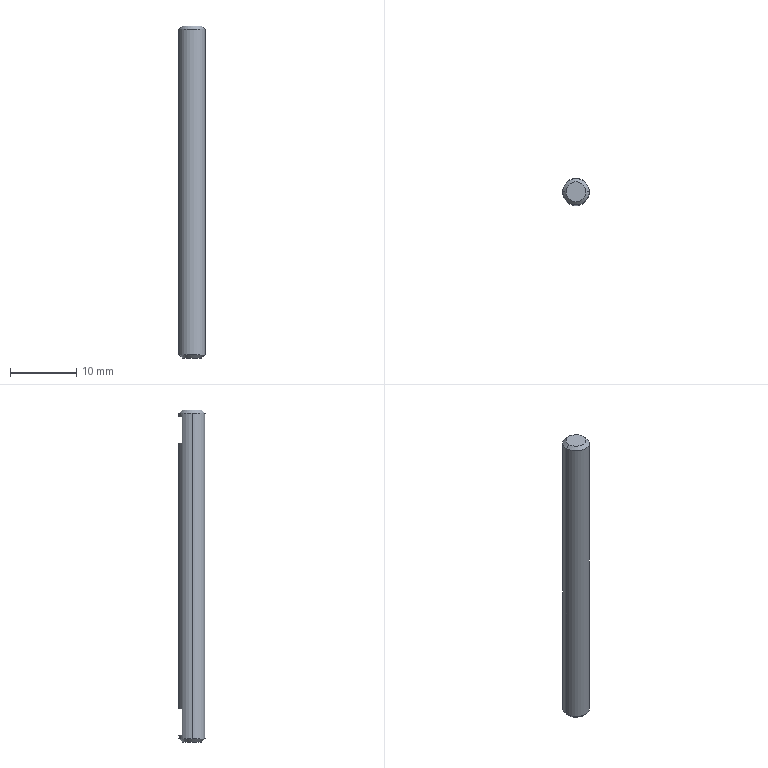Part | SolidWorks | features Chamfer 1, Extrusion 1, ICE 1 | 1 solid | 14 faces | box 4 x 4 x 50 mm | volume 618.186 mm3 | plane 8 | cone 4 | cylinder 2 | commonest cylinder face diameters 4 x2
STEP:
#1=CARTESIAN_POINT('',(-1.5,0.,-25.));
#2=VERTEX_POINT('',#1);
#3=CARTESIAN_POINT('',(1.5,0.,-25.));
#4=VERTEX_POINT('',#3);
#5=CARTESIAN_POINT('',(0.,0.,-25.));
#6=DIRECTION('',(0.,0.,-1.));
#7=DIRECTION('',(1.,0.,0.));
#8=AXIS2_PLACEMENT_3D('',#5,#6,#7);
#9=CIRCLE('',#8,1.5);
#10=EDGE_CURVE('',#2,#4,#9,.T.);
#11=ORIENTED_EDGE('',*,*,#10,.F.);
#12=CARTESIAN_POINT('',(-2.,0.,-24.5));
#13=VERTEX_POINT('',#12);
#14=CARTESIAN_POINT('',(-2.,0.,-24.5));
#15=DIRECTION('',(-0.7071,0.,0.7071));
#16=VECTOR('',#15,1000.);
#17=LINE('',#14,#16);
#18=EDGE_CURVE('',#2,#13,#17,.T.);
#19=ORIENTED_EDGE('',*,*,#18,.T.);
#20=CARTESIAN_POINT('',(2.,0.,-24.5));
#21=VERTEX_POINT('',#20);
#22=CARTESIAN_POINT('',(0.,0.,-24.5));
#23=DIRECTION('',(0.,0.,1.));
#24=DIRECTION('',(1.,0.,0.));
#25=AXIS2_PLACEMENT_3D('',#22,#23,#24);
#26=CIRCLE('',#25,2.);
#27=EDGE_CURVE('',#21,#13,#26,.T.);
#28=ORIENTED_EDGE('',*,*,#27,.F.);
#29=CARTESIAN_POINT('',(2.,0.,-24.5));
#30=DIRECTION('',(0.7071,0.,0.7071));
#31=VECTOR('',#30,1000.);
#32=LINE('',#29,#31);
#33=EDGE_CURVE('',#4,#21,#32,.T.);
#34=ORIENTED_EDGE('',*,*,#33,.F.);
#35=EDGE_LOOP('',(#11,#19,#28,#34));
#36=FACE_OUTER_BOUND('',#35,.T.);
#37=CARTESIAN_POINT('',(0.,0.,-24.5));
#38=DIRECTION('',(0.,0.,1.));
#39=DIRECTION('',(1.,0.,0.));
#40=AXIS2_PLACEMENT_3D('',#37,#38,#39);
#41=CONICAL_SURFACE('',#40,2.,0.7854);
#42=ADVANCED_FACE('',(#36),#41,.T.);
#43=CARTESIAN_POINT('',(1.5,0.,25.));
#44=VERTEX_POINT('',#43);
#45=CARTESIAN_POINT('',(-1.5,0.,25.));
#46=VERTEX_POINT('',#45);
#47=CARTESIAN_POINT('',(0.,0.,25.));
#48=DIRECTION('',(0.,0.,1.));
#49=DIRECTION('',(1.,0.,0.));
#50=AXIS2_PLACEMENT_3D('',#47,#48,#49);
#51=CIRCLE('',#50,1.5);
#52=EDGE_CURVE('',#44,#46,#51,.T.);
#53=ORIENTED_EDGE('',*,*,#52,.F.);
#54=CARTESIAN_POINT('',(2.,0.,24.5));
#55=VERTEX_POINT('',#54);
#56=CARTESIAN_POINT('',(1.5,0.,25.));
#57=DIRECTION('',(0.7071,0.,-0.7071));
#58=VECTOR('',#57,1000.);
#59=LINE('',#56,#58);
#60=EDGE_CURVE('',#44,#55,#59,.T.);
#61=ORIENTED_EDGE('',*,*,#60,.T.);
#62=CARTESIAN_POINT('',(-2.,0.,24.5));
#63=VERTEX_POINT('',#62);
#64=CARTESIAN_POINT('',(0.,0.,24.5));
#65=DIRECTION('',(0.,0.,-1.));
#66=DIRECTION('',(1.,0.,0.));
#67=AXIS2_PLACEMENT_3D('',#64,#65,#66);
#68=CIRCLE('',#67,2.);
#69=EDGE_CURVE('',#63,#55,#68,.T.);
#70=ORIENTED_EDGE('',*,*,#69,.F.);
#71=CARTESIAN_POINT('',(-1.5,0.,25.));
#72=DIRECTION('',(-0.7071,0.,-0.7071));
#73=VECTOR('',#72,1000.);
#74=LINE('',#71,#73);
#75=EDGE_CURVE('',#46,#63,#74,.T.);
#76=ORIENTED_EDGE('',*,*,#75,.F.);
#77=EDGE_LOOP('',(#53,#61,#70,#76));
#78=FACE_OUTER_BOUND('',#77,.T.);
#79=CARTESIAN_POINT('',(0.,0.,25.));
#80=DIRECTION('',(0.,0.,-1.));
#81=DIRECTION('',(-1.,0.,0.));
#82=AXIS2_PLACEMENT_3D('',#79,#80,#81);
#83=CONICAL_SURFACE('',#82,1.5,0.7854);
#84=ADVANCED_FACE('',(#78),#83,.T.);
#85=CARTESIAN_POINT('',(1.323,1.5,-20.));
#86=VERTEX_POINT('',#85);
#87=CARTESIAN_POINT('',(1.323,1.5,-24.));
#88=VERTEX_POINT('',#87);
#89=CARTESIAN_POINT('',(1.323,1.5,25.));
#90=DIRECTION('',(0.,0.,-1.));
#91=VECTOR('',#90,1000.);
#92=LINE('',#89,#91);
#93=EDGE_CURVE('',#86,#88,#92,.T.);
#94=ORIENTED_EDGE('',*,*,#93,.F.);
#95=CARTESIAN_POINT('',(-1.323,1.5,-20.));
#96=VERTEX_POINT('',#95);
#97=CARTESIAN_POINT('',(0.,0.,-20.));
#98=DIRECTION('',(0.,0.,1.));
#99=DIRECTION('',(1.,0.,0.));
#100=AXIS2_PLACEMENT_3D('',#97,#98,#99);
#101=CIRCLE('',#100,2.);
#102=EDGE_CURVE('',#86,#96,#101,.T.);
#103=ORIENTED_EDGE('',*,*,#102,.T.);
#104=CARTESIAN_POINT('',(-1.323,1.5,-24.));
#105=VERTEX_POINT('',#104);
#106=CARTESIAN_POINT('',(-1.323,1.5,25.));
#107=DIRECTION('',(0.,0.,1.));
#108=VECTOR('',#107,1000.);
#109=LINE('',#106,#108);
#110=EDGE_CURVE('',#105,#96,#109,.T.);
#111=ORIENTED_EDGE('',*,*,#110,.F.);
#112=CARTESIAN_POINT('',(0.,0.,-24.));
#113=DIRECTION('',(0.,0.,-1.));
#114=DIRECTION('',(-1.,0.,0.));
#115=AXIS2_PLACEMENT_3D('',#112,#113,#114);
#116=CIRCLE('',#115,2.);
#117=EDGE_CURVE('',#105,#88,#116,.T.);
#118=ORIENTED_EDGE('',*,*,#117,.T.);
#119=EDGE_LOOP('',(#94,#103,#111,#118));
#120=FACE_BOUND('',#119,.T.);
#121=CARTESIAN_POINT('',(1.323,1.5,24.));
#122=VERTEX_POINT('',#121);
#123=CARTESIAN_POINT('',(1.323,1.5,20.));
#124=VERTEX_POINT('',#123);
#125=CARTESIAN_POINT('',(1.323,1.5,25.));
#126=DIRECTION('',(0.,0.,-1.));
#127=VECTOR('',#126,1000.);
#128=LINE('',#125,#127);
#129=EDGE_CURVE('',#122,#124,#128,.T.);
#130=ORIENTED_EDGE('',*,*,#129,.F.);
#131=CARTESIAN_POINT('',(-1.323,1.5,24.));
#132=VERTEX_POINT('',#131);
#133=CARTESIAN_POINT('',(0.,0.,24.));
#134=DIRECTION('',(0.,0.,1.));
#135=DIRECTION('',(1.,0.,0.));
#136=AXIS2_PLACEMENT_3D('',#133,#134,#135);
#137=CIRCLE('',#136,2.);
#138=EDGE_CURVE('',#122,#132,#137,.T.);
#139=ORIENTED_EDGE('',*,*,#138,.T.);
#140=CARTESIAN_POINT('',(-1.323,1.5,20.));
#141=VERTEX_POINT('',#140);
#142=CARTESIAN_POINT('',(-1.323,1.5,25.));
#143=DIRECTION('',(0.,0.,1.));
#144=VECTOR('',#143,1000.);
#145=LINE('',#142,#144);
#146=EDGE_CURVE('',#141,#132,#145,.T.);
#147=ORIENTED_EDGE('',*,*,#146,.F.);
#148=CARTESIAN_POINT('',(0.,0.,20.));
#149=DIRECTION('',(0.,0.,-1.));
#150=DIRECTION('',(-1.,0.,0.));
#151=AXIS2_PLACEMENT_3D('',#148,#149,#150);
#152=CIRCLE('',#151,2.);
#153=EDGE_CURVE('',#141,#124,#152,.T.);
#154=ORIENTED_EDGE('',*,*,#153,.T.);
#155=EDGE_LOOP('',(#130,#139,#147,#154));
#156=FACE_BOUND('',#155,.T.);
#157=ORIENTED_EDGE('',*,*,#69,.T.);
#158=CARTESIAN_POINT('',(2.,0.,25.));
#159=DIRECTION('',(0.,0.,-1.));
#160=VECTOR('',#159,1000.);
#161=LINE('',#158,#160);
#162=EDGE_CURVE('',#55,#21,#161,.T.);
#163=ORIENTED_EDGE('',*,*,#162,.T.);
#164=ORIENTED_EDGE('',*,*,#27,.T.);
#165=CARTESIAN_POINT('',(-2.,0.,25.));
#166=DIRECTION('',(0.,0.,-1.));
#167=VECTOR('',#166,1000.);
#168=LINE('',#165,#167);
#169=EDGE_CURVE('',#63,#13,#168,.T.);
#170=ORIENTED_EDGE('',*,*,#169,.F.);
#171=EDGE_LOOP('',(#157,#163,#164,#170));
#172=FACE_OUTER_BOUND('',#171,.T.);
#173=CARTESIAN_POINT('',(0.,0.,25.));
#174=DIRECTION('',(0.,0.,-1.));
#175=DIRECTION('',(-1.,0.,0.));
#176=AXIS2_PLACEMENT_3D('',#173,#174,#175);
#177=CYLINDRICAL_SURFACE('',#176,2.);
#178=ADVANCED_FACE('',(#120,#156,#172),#177,.T.);
#179=ORIENTED_EDGE('',*,*,#162,.F.);
#180=CARTESIAN_POINT('',(0.,0.,24.5));
#181=DIRECTION('',(0.,0.,-1.));
#182=DIRECTION('',(1.,0.,0.));
#183=AXIS2_PLACEMENT_3D('',#180,#181,#182);
#184=CIRCLE('',#183,2.);
#185=EDGE_CURVE('',#55,#63,#184,.T.);
#186=ORIENTED_EDGE('',*,*,#185,.T.);
#187=ORIENTED_EDGE('',*,*,#169,.T.);
#188=CARTESIAN_POINT('',(0.,0.,-24.5));
#189=DIRECTION('',(0.,0.,1.));
#190=DIRECTION('',(1.,0.,0.));
#191=AXIS2_PLACEMENT_3D('',#188,#189,#190);
#192=CIRCLE('',#191,2.);
#193=EDGE_CURVE('',#13,#21,#192,.T.);
#194=ORIENTED_EDGE('',*,*,#193,.T.);
#195=EDGE_LOOP('',(#179,#186,#187,#194));
#196=FACE_OUTER_BOUND('',#195,.T.);
#197=CARTESIAN_POINT('',(0.,0.,25.));
#198=DIRECTION('',(0.,0.,-1.));
#199=DIRECTION('',(-1.,0.,0.));
#200=AXIS2_PLACEMENT_3D('',#197,#198,#199);
#201=CYLINDRICAL_SURFACE('',#200,2.);
#202=ADVANCED_FACE('',(#196),#201,.T.);
#203=CARTESIAN_POINT('',(0.,0.,25.));
#204=DIRECTION('',(0.,0.,1.));
#205=DIRECTION('',(1.,0.,0.));
#206=AXIS2_PLACEMENT_3D('',#203,#204,#205);
#207=CIRCLE('',#206,1.5);
#208=EDGE_CURVE('',#46,#44,#207,.T.);
#209=ORIENTED_EDGE('',*,*,#208,.T.);
#210=ORIENTED_EDGE('',*,*,#52,.T.);
#211=EDGE_LOOP('',(#209,#210));
#212=FACE_OUTER_BOUND('',#211,.T.);
#213=CARTESIAN_POINT('',(0.,0.,25.));
#214=DIRECTION('',(0.,0.,1.));
#215=DIRECTION('',(1.,0.,0.));
#216=AXIS2_PLACEMENT_3D('',#213,#214,#215);
#217=PLANE('',#216);
#218=ADVANCED_FACE('',(#212),#217,.T.);
#219=CARTESIAN_POINT('',(0.,0.,-25.));
#220=DIRECTION('',(0.,0.,-1.));
#221=DIRECTION('',(1.,0.,0.));
#222=AXIS2_PLACEMENT_3D('',#219,#220,#221);
#223=CIRCLE('',#222,1.5);
#224=EDGE_CURVE('',#4,#2,#223,.T.);
#225=ORIENTED_EDGE('',*,*,#224,.T.);
#226=ORIENTED_EDGE('',*,*,#10,.T.);
#227=EDGE_LOOP('',(#225,#226));
#228=FACE_OUTER_BOUND('',#227,.T.);
#229=CARTESIAN_POINT('',(0.,0.,-25.));
#230=DIRECTION('',(0.,0.,1.));
#231=DIRECTION('',(1.,0.,0.));
#232=AXIS2_PLACEMENT_3D('',#229,#230,#231);
#233=PLANE('',#232);
#234=ADVANCED_FACE('',(#228),#233,.F.);
#235=CARTESIAN_POINT('',(7.709,1.5,24.));
#236=DIRECTION('',(1.,0.,0.));
#237=VECTOR('',#236,1000.);
#238=LINE('',#235,#237);
#239=EDGE_CURVE('',#132,#122,#238,.T.);
#240=ORIENTED_EDGE('',*,*,#239,.F.);
#241=ORIENTED_EDGE('',*,*,#138,.F.);
#242=EDGE_LOOP('',(#240,#241));
#243=FACE_OUTER_BOUND('',#242,.T.);
#244=CARTESIAN_POINT('',(7.709,1.5,24.));
#245=DIRECTION('',(0.,0.,1.));
#246=DIRECTION('',(1.,0.,0.));
#247=AXIS2_PLACEMENT_3D('',#244,#245,#246);
#248=PLANE('',#247);
#249=ADVANCED_FACE('',(#243),#248,.F.);
#250=CARTESIAN_POINT('',(7.709,1.5,20.));
#251=DIRECTION('',(-1.,0.,0.));
#252=VECTOR('',#251,1000.);
#253=LINE('',#250,#252);
#254=EDGE_CURVE('',#124,#141,#253,.T.);
#255=ORIENTED_EDGE('',*,*,#254,.F.);
#256=ORIENTED_EDGE('',*,*,#153,.F.);
#257=EDGE_LOOP('',(#255,#256));
#258=FACE_OUTER_BOUND('',#257,.T.);
#259=CARTESIAN_POINT('',(7.709,1.5,20.));
#260=DIRECTION('',(0.,0.,-1.));
#261=DIRECTION('',(-1.,0.,0.));
#262=AXIS2_PLACEMENT_3D('',#259,#260,#261);
#263=PLANE('',#262);
#264=ADVANCED_FACE('',(#258),#263,.F.);
#265=ORIENTED_EDGE('',*,*,#129,.T.);
#266=ORIENTED_EDGE('',*,*,#254,.T.);
#267=ORIENTED_EDGE('',*,*,#146,.T.);
#268=ORIENTED_EDGE('',*,*,#239,.T.);
#269=EDGE_LOOP('',(#265,#266,#267,#268));
#270=FACE_OUTER_BOUND('',#269,.T.);
#271=CARTESIAN_POINT('',(7.709,1.5,20.));
#272=DIRECTION('',(0.,1.,0.));
#273=DIRECTION('',(0.,0.,1.));
#274=AXIS2_PLACEMENT_3D('',#271,#272,#273);
#275=PLANE('',#274);
#276=ADVANCED_FACE('',(#270),#275,.T.);
#277=CARTESIAN_POINT('',(5.032,1.5,-20.));
#278=DIRECTION('',(1.,0.,0.));
#279=VECTOR('',#278,1000.);
#280=LINE('',#277,#279);
#281=EDGE_CURVE('',#96,#86,#280,.T.);
#282=ORIENTED_EDGE('',*,*,#281,.F.);
#283=ORIENTED_EDGE('',*,*,#102,.F.);
#284=EDGE_LOOP('',(#282,#283));
#285=FACE_OUTER_BOUND('',#284,.T.);
#286=CARTESIAN_POINT('',(5.032,1.5,-20.));
#287=DIRECTION('',(0.,0.,1.));
#288=DIRECTION('',(1.,0.,0.));
#289=AXIS2_PLACEMENT_3D('',#286,#287,#288);
#290=PLANE('',#289);
#291=ADVANCED_FACE('',(#285),#290,.F.);
#292=CARTESIAN_POINT('',(5.032,1.5,-24.));
#293=DIRECTION('',(-1.,0.,0.));
#294=VECTOR('',#293,1000.);
#295=LINE('',#292,#294);
#296=EDGE_CURVE('',#88,#105,#295,.T.);
#297=ORIENTED_EDGE('',*,*,#296,.F.);
#298=ORIENTED_EDGE('',*,*,#117,.F.);
#299=EDGE_LOOP('',(#297,#298));
#300=FACE_OUTER_BOUND('',#299,.T.);
#301=CARTESIAN_POINT('',(5.032,1.5,-24.));
#302=DIRECTION('',(0.,0.,-1.));
#303=DIRECTION('',(-1.,0.,0.));
#304=AXIS2_PLACEMENT_3D('',#301,#302,#303);
#305=PLANE('',#304);
#306=ADVANCED_FACE('',(#300),#305,.F.);
#307=ORIENTED_EDGE('',*,*,#93,.T.);
#308=ORIENTED_EDGE('',*,*,#296,.T.);
#309=ORIENTED_EDGE('',*,*,#110,.T.);
#310=ORIENTED_EDGE('',*,*,#281,.T.);
#311=EDGE_LOOP('',(#307,#308,#309,#310));
#312=FACE_OUTER_BOUND('',#311,.T.);
#313=CARTESIAN_POINT('',(5.032,1.5,-24.));
#314=DIRECTION('',(0.,1.,0.));
#315=DIRECTION('',(0.,0.,1.));
#316=AXIS2_PLACEMENT_3D('',#313,#314,#315);
#317=PLANE('',#316);
#318=ADVANCED_FACE('',(#312),#317,.T.);
#319=ORIENTED_EDGE('',*,*,#60,.F.);
#320=ORIENTED_EDGE('',*,*,#208,.F.);
#321=ORIENTED_EDGE('',*,*,#75,.T.);
#322=ORIENTED_EDGE('',*,*,#185,.F.);
#323=EDGE_LOOP('',(#319,#320,#321,#322));
#324=FACE_OUTER_BOUND('',#323,.T.);
#325=CARTESIAN_POINT('',(0.,0.,25.));
#326=DIRECTION('',(0.,0.,-1.));
#327=DIRECTION('',(-1.,0.,0.));
#328=AXIS2_PLACEMENT_3D('',#325,#326,#327);
#329=CONICAL_SURFACE('',#328,1.5,0.7854);
#330=ADVANCED_FACE('',(#324),#329,.T.);
#331=ORIENTED_EDGE('',*,*,#18,.F.);
#332=ORIENTED_EDGE('',*,*,#224,.F.);
#333=ORIENTED_EDGE('',*,*,#33,.T.);
#334=ORIENTED_EDGE('',*,*,#193,.F.);
#335=EDGE_LOOP('',(#331,#332,#333,#334));
#336=FACE_OUTER_BOUND('',#335,.T.);
#337=CARTESIAN_POINT('',(0.,0.,-24.5));
#338=DIRECTION('',(0.,0.,1.));
#339=DIRECTION('',(1.,0.,0.));
#340=AXIS2_PLACEMENT_3D('',#337,#338,#339);
#341=CONICAL_SURFACE('',#340,2.,0.7854);
#342=ADVANCED_FACE('',(#336),#341,.T.);
#343=CLOSED_SHELL('',(#42,#84,#178,#202,#218,#234,#249,#264,#276,#291,#306,#318,#330,#342));
#344=MANIFOLD_SOLID_BREP('',#343);
#345=CARTESIAN_POINT('',(0.,0.,0.));
#346=DIRECTION('',(0.,0.,1.));
#347=DIRECTION('',(1.,0.,0.));
#348=AXIS2_PLACEMENT_3D('',#345,#346,#347);
#349=(LENGTH_UNIT()NAMED_UNIT(*)SI_UNIT(.MILLI.,.METRE.));
#350=UNCERTAINTY_MEASURE_WITH_UNIT(LENGTH_MEASURE(0.00001),#349,'','');
#351=(NAMED_UNIT(*)PLANE_ANGLE_UNIT()SI_UNIT($,.RADIAN.));
#352=(NAMED_UNIT(*)SI_UNIT($,.STERADIAN.)SOLID_ANGLE_UNIT());
#353=(GEOMETRIC_REPRESENTATION_CONTEXT(3)GLOBAL_UNCERTAINTY_ASSIGNED_CONTEXT((#350))GLOBAL_UNIT_ASSIGNED_CONTEXT((#349,#351,#352))REPRESENTATION_CONTEXT('',''));
#354=ADVANCED_BREP_SHAPE_REPRESENTATION('',(#344,#348),#353);